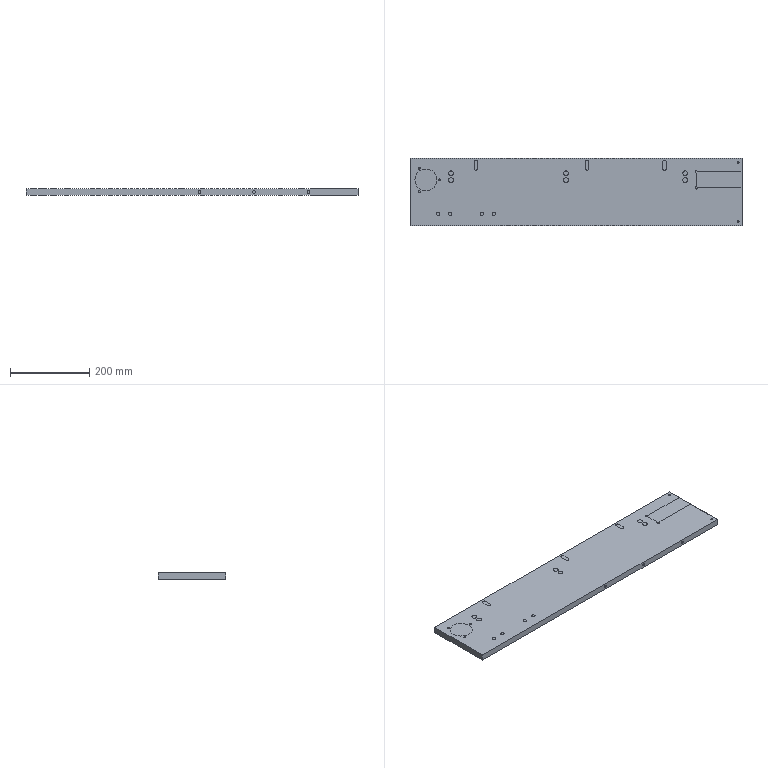CAM job | NX | 3-axis milling, drilling | part box 836 x 170 x 16 mm | stock box 836 x 170 x 16 mm
Tools:
number,name,description,diameter,corner_radius,flute_length,length,flutes
0,D6点孔钻,Drilling Tool,10.0,0.0,5.0,40.0,2
0,D21R0.8圆鼻飞刀,Milling Tool-5 Parameters,25.0,0.8,50.0,50.0,2
0,D8平底刀,Milling Tool-5 Parameters,8.0,0.0,20.0,23.0,4
0,D4平底刀,Milling Tool-5 Parameters,4.5,0.0,20.0,40.0,3
0,D10平底刀,Milling Tool-5 Parameters,10.0,0.0,22.0,25.0,4
0,D17R0.8圆鼻飞刀,Milling Tool-5 Parameters,17.0,0.8,60.0,60.0,2
0,D6倒角刀,Milling Tool-5 Parameters,1.6,0.0,2.7,2.7,2
Operations:
program,operation,operation_type,tool,method,geometry_group,spindle_rpm,surface_speed,feed_per_tooth,feed_cut,feed_plunge,cut_length_mm,path_length_mm,cut_time_min,machine_time_min
0153.NC,G81点孔,Operation,D6点孔钻,METHOD,WORKPIECE---A,1500.0,47.0,0.0333,100.0,0.0,48.0,1526.911,0.48,0.6279
0153.NC,孔铣开粗_2,CylinderMilling,D17R0.8圆鼻飞刀,METHOD,WORKPIECE---A,2000.0,106.0,0.325,1300.0,80.0,4399.264,4615.064,3.387,3.408
0153.NC,孔铣开粗,CylinderMilling,D21R0.8圆鼻飞刀,METHOD,WORKPIECE---A,1700.0,133.0,0.4412,1500.0,80.0,8137.543,8353.343,5.429,5.451
0153.NC,等高外形,ZLevelMilling,D21R0.8圆鼻飞刀,METHOD,WORKPIECE---A,1500.0,117.0,0.4333,1300.0,80.0,15430.143,15710.749,12.123,12.151
0153.NC,等高外形_1,ZLevelMilling,D8平底刀,METHOD,WORKPIECE---A,2600.0,65.0,0.1442,1500.0,80.0,14944.122,15222.526,10.004,10.032
0153.NC,等高外形_2,ZLevelMilling,D8平底刀,METHOD,WORKPIECE---A,2600.0,65.0,0.1442,1500.0,80.0,8551.368,9674.426,5.702,5.814
0153.NC,孔铣开粗_1,CylinderMilling,D8平底刀,METHOD,WORKPIECE---A,2600.0,65.0,0.0962,1000.0,80.0,2869.116,5045.642,2.875,3.093
0153.NC,等高清角,ZLevelMilling,D4平底刀,METHOD,WORKPIECE---A,3000.0,42.0,0.1111,1000.0,80.0,2604.298,3107.687,2.708,2.759
0153.NC,2D边界补正,PlanarMilling,D10平底刀,METHOD,WORKPIECE---A,3000.0,94.0,0.0417,500.0,80.0,160.203,392.203,0.3251,0.3483
0153.NC,2D边界补正_COPY,PlanarMilling,D10平底刀,METHOD,WORKPIECE---A,3000.0,94.0,0.0417,500.0,80.0,268.632,500.632,0.557,0.5802
0153.NC,G81点孔_1,Operation,D6点孔钻,METHOD,MCS---A,1500.0,47.0,0.02,60.0,0.0,18.0,899.685,0.3,0.3882
0153.NC,边界倒角,PlanarMilling,D6倒角刀,METHOD,MCS---A,3000.0,15.0,0.1333,800.0,80.0,126.419,1209.434,0.1606,0.2689
0153.NC,边界倒角_1,PlanarMilling,D6倒角刀,METHOD,MCS---A,3000.0,15.0,0.1333,800.0,80.0,414.195,1640.055,0.5194,0.6419